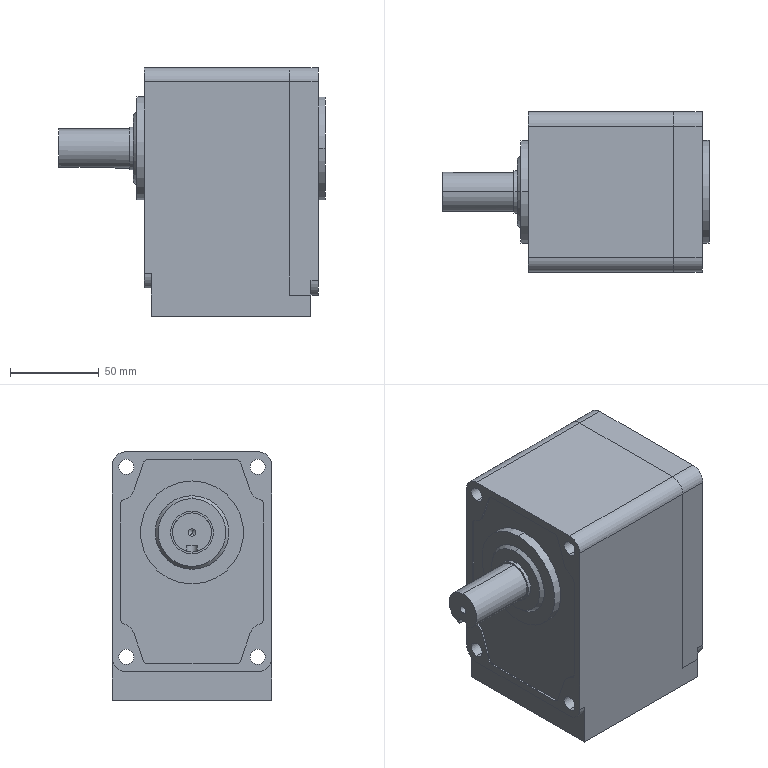Part | STEP file | 0229_Z_5IK40AW-GAL20J_1 | 2 solids | 107 faces | box 150 x 90 x 140 mm | volume 1226880 mm3 | cylinder 59 | plane 44 | cone 4 | commonest cylinder face diameters 6 x17 8.5 x16 16 x8 18 x8 58 x4 4.2 x2